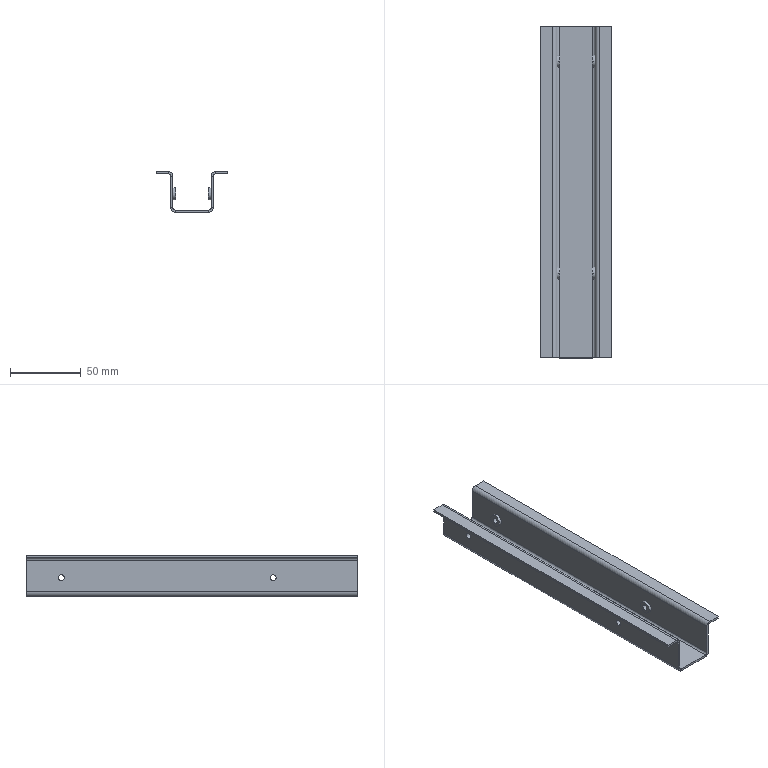Part | SolidWorks | features ICE 2, 3DProfileFeature 1, FlatPattern 1, HoleWzd 1, MirrorPattern 1, SMBaseFlange 1, SheetMetal 1 | 1 solid | 58 faces | box 50 x 235 x 28.5 mm | volume 35580 mm3 | plane 34 | cylinder 24 | commonest cylinder face diameters 4.2 x8 8.7 x8 3 x4 6 x4
STEP:
#1=CARTESIAN_POINT('',(15.,225.,-11.9));
#2=VERTEX_POINT('',#1);
#3=CARTESIAN_POINT('',(15.,225.,-16.1));
#4=VERTEX_POINT('',#3);
#5=CARTESIAN_POINT('',(15.,225.,-14.));
#6=DIRECTION('',(1.,0.,0.));
#7=DIRECTION('',(0.,0.,-1.));
#8=AXIS2_PLACEMENT_3D('',#5,#6,#7);
#9=CIRCLE('',#8,2.1);
#10=EDGE_CURVE('',#2,#4,#9,.T.);
#11=ORIENTED_EDGE('',*,*,#10,.T.);
#12=CARTESIAN_POINT('',(11.5,225.,-16.1));
#13=VERTEX_POINT('',#12);
#14=CARTESIAN_POINT('',(-15.,225.,-16.1));
#15=DIRECTION('',(-1.,0.,0.));
#16=VECTOR('',#15,1000.);
#17=LINE('',#14,#16);
#18=EDGE_CURVE('',#4,#13,#17,.T.);
#19=ORIENTED_EDGE('',*,*,#18,.T.);
#20=CARTESIAN_POINT('',(11.5,225.,-11.9));
#21=VERTEX_POINT('',#20);
#22=CARTESIAN_POINT('',(11.5,225.,-14.));
#23=DIRECTION('',(-1.,0.,0.));
#24=DIRECTION('',(0.,0.,1.));
#25=AXIS2_PLACEMENT_3D('',#22,#23,#24);
#26=CIRCLE('',#25,2.1);
#27=EDGE_CURVE('',#13,#21,#26,.T.);
#28=ORIENTED_EDGE('',*,*,#27,.T.);
#29=CARTESIAN_POINT('',(-15.,225.,-11.9));
#30=DIRECTION('',(-1.,0.,0.));
#31=VECTOR('',#30,1000.);
#32=LINE('',#29,#31);
#33=EDGE_CURVE('',#2,#21,#32,.T.);
#34=ORIENTED_EDGE('',*,*,#33,.F.);
#35=EDGE_LOOP('',(#11,#19,#28,#34));
#36=FACE_OUTER_BOUND('',#35,.T.);
#37=CARTESIAN_POINT('',(-15.,225.,-14.));
#38=DIRECTION('',(-1.,0.,0.));
#39=DIRECTION('',(0.,0.,1.));
#40=AXIS2_PLACEMENT_3D('',#37,#38,#39);
#41=CYLINDRICAL_SURFACE('',#40,2.1);
#42=ADVANCED_FACE('',(#36),#41,.F.);
#43=CARTESIAN_POINT('',(-11.5,225.,-11.9));
#44=VERTEX_POINT('',#43);
#45=CARTESIAN_POINT('',(-11.5,225.,-16.1));
#46=VERTEX_POINT('',#45);
#47=CARTESIAN_POINT('',(-11.5,225.,-14.));
#48=DIRECTION('',(1.,0.,0.));
#49=DIRECTION('',(0.,0.,-1.));
#50=AXIS2_PLACEMENT_3D('',#47,#48,#49);
#51=CIRCLE('',#50,2.1);
#52=EDGE_CURVE('',#44,#46,#51,.T.);
#53=ORIENTED_EDGE('',*,*,#52,.T.);
#54=CARTESIAN_POINT('',(-15.,225.,-16.1));
#55=VERTEX_POINT('',#54);
#56=CARTESIAN_POINT('',(-15.,225.,-16.1));
#57=DIRECTION('',(-1.,0.,0.));
#58=VECTOR('',#57,1000.);
#59=LINE('',#56,#58);
#60=EDGE_CURVE('',#46,#55,#59,.T.);
#61=ORIENTED_EDGE('',*,*,#60,.T.);
#62=CARTESIAN_POINT('',(-15.,225.,-11.9));
#63=VERTEX_POINT('',#62);
#64=CARTESIAN_POINT('',(-15.,225.,-14.));
#65=DIRECTION('',(-1.,0.,0.));
#66=DIRECTION('',(0.,0.,1.));
#67=AXIS2_PLACEMENT_3D('',#64,#65,#66);
#68=CIRCLE('',#67,2.1);
#69=EDGE_CURVE('',#55,#63,#68,.T.);
#70=ORIENTED_EDGE('',*,*,#69,.T.);
#71=CARTESIAN_POINT('',(-15.,225.,-11.9));
#72=DIRECTION('',(-1.,0.,0.));
#73=VECTOR('',#72,1000.);
#74=LINE('',#71,#73);
#75=EDGE_CURVE('',#44,#63,#74,.T.);
#76=ORIENTED_EDGE('',*,*,#75,.F.);
#77=EDGE_LOOP('',(#53,#61,#70,#76));
#78=FACE_OUTER_BOUND('',#77,.T.);
#79=CARTESIAN_POINT('',(-15.,225.,-14.));
#80=DIRECTION('',(-1.,0.,0.));
#81=DIRECTION('',(0.,0.,1.));
#82=AXIS2_PLACEMENT_3D('',#79,#80,#81);
#83=CYLINDRICAL_SURFACE('',#82,2.1);
#84=ADVANCED_FACE('',(#78),#83,.F.);
#85=CARTESIAN_POINT('',(-11.5,75.,-11.9));
#86=VERTEX_POINT('',#85);
#87=CARTESIAN_POINT('',(-11.5,75.,-16.1));
#88=VERTEX_POINT('',#87);
#89=CARTESIAN_POINT('',(-11.5,75.,-14.));
#90=DIRECTION('',(1.,0.,0.));
#91=DIRECTION('',(0.,0.,-1.));
#92=AXIS2_PLACEMENT_3D('',#89,#90,#91);
#93=CIRCLE('',#92,2.1);
#94=EDGE_CURVE('',#86,#88,#93,.T.);
#95=ORIENTED_EDGE('',*,*,#94,.T.);
#96=CARTESIAN_POINT('',(-15.,75.,-16.1));
#97=VERTEX_POINT('',#96);
#98=CARTESIAN_POINT('',(-15.,75.,-16.1));
#99=DIRECTION('',(-1.,0.,0.));
#100=VECTOR('',#99,1000.);
#101=LINE('',#98,#100);
#102=EDGE_CURVE('',#88,#97,#101,.T.);
#103=ORIENTED_EDGE('',*,*,#102,.T.);
#104=CARTESIAN_POINT('',(-15.,75.,-11.9));
#105=VERTEX_POINT('',#104);
#106=CARTESIAN_POINT('',(-15.,75.,-14.));
#107=DIRECTION('',(-1.,0.,0.));
#108=DIRECTION('',(0.,0.,1.));
#109=AXIS2_PLACEMENT_3D('',#106,#107,#108);
#110=CIRCLE('',#109,2.1);
#111=EDGE_CURVE('',#97,#105,#110,.T.);
#112=ORIENTED_EDGE('',*,*,#111,.T.);
#113=CARTESIAN_POINT('',(-15.,75.,-11.9));
#114=DIRECTION('',(-1.,0.,0.));
#115=VECTOR('',#114,1000.);
#116=LINE('',#113,#115);
#117=EDGE_CURVE('',#86,#105,#116,.T.);
#118=ORIENTED_EDGE('',*,*,#117,.F.);
#119=EDGE_LOOP('',(#95,#103,#112,#118));
#120=FACE_OUTER_BOUND('',#119,.T.);
#121=CARTESIAN_POINT('',(-15.,75.,-14.));
#122=DIRECTION('',(-1.,0.,0.));
#123=DIRECTION('',(0.,0.,1.));
#124=AXIS2_PLACEMENT_3D('',#121,#122,#123);
#125=CYLINDRICAL_SURFACE('',#124,2.1);
#126=ADVANCED_FACE('',(#120),#125,.F.);
#127=CARTESIAN_POINT('',(15.,75.,-11.9));
#128=VERTEX_POINT('',#127);
#129=CARTESIAN_POINT('',(15.,75.,-16.1));
#130=VERTEX_POINT('',#129);
#131=CARTESIAN_POINT('',(15.,75.,-14.));
#132=DIRECTION('',(1.,0.,0.));
#133=DIRECTION('',(0.,0.,-1.));
#134=AXIS2_PLACEMENT_3D('',#131,#132,#133);
#135=CIRCLE('',#134,2.1);
#136=EDGE_CURVE('',#128,#130,#135,.T.);
#137=ORIENTED_EDGE('',*,*,#136,.T.);
#138=CARTESIAN_POINT('',(11.5,75.,-16.1));
#139=VERTEX_POINT('',#138);
#140=CARTESIAN_POINT('',(-15.,75.,-16.1));
#141=DIRECTION('',(-1.,0.,0.));
#142=VECTOR('',#141,1000.);
#143=LINE('',#140,#142);
#144=EDGE_CURVE('',#130,#139,#143,.T.);
#145=ORIENTED_EDGE('',*,*,#144,.T.);
#146=CARTESIAN_POINT('',(11.5,75.,-11.9));
#147=VERTEX_POINT('',#146);
#148=CARTESIAN_POINT('',(11.5,75.,-14.));
#149=DIRECTION('',(-1.,0.,0.));
#150=DIRECTION('',(0.,0.,1.));
#151=AXIS2_PLACEMENT_3D('',#148,#149,#150);
#152=CIRCLE('',#151,2.1);
#153=EDGE_CURVE('',#139,#147,#152,.T.);
#154=ORIENTED_EDGE('',*,*,#153,.T.);
#155=CARTESIAN_POINT('',(-15.,75.,-11.9));
#156=DIRECTION('',(-1.,0.,0.));
#157=VECTOR('',#156,1000.);
#158=LINE('',#155,#157);
#159=EDGE_CURVE('',#128,#147,#158,.T.);
#160=ORIENTED_EDGE('',*,*,#159,.F.);
#161=EDGE_LOOP('',(#137,#145,#154,#160));
#162=FACE_OUTER_BOUND('',#161,.T.);
#163=CARTESIAN_POINT('',(-15.,75.,-14.));
#164=DIRECTION('',(-1.,0.,0.));
#165=DIRECTION('',(0.,0.,1.));
#166=AXIS2_PLACEMENT_3D('',#163,#164,#165);
#167=CYLINDRICAL_SURFACE('',#166,2.1);
#168=ADVANCED_FACE('',(#162),#167,.F.);
#169=CARTESIAN_POINT('',(11.5,75.,-18.35));
#170=VERTEX_POINT('',#169);
#171=CARTESIAN_POINT('',(11.5,75.,-9.65));
#172=VERTEX_POINT('',#171);
#173=CARTESIAN_POINT('',(11.5,75.,-14.));
#174=DIRECTION('',(1.,0.,0.));
#175=DIRECTION('',(0.,0.,-1.));
#176=AXIS2_PLACEMENT_3D('',#173,#174,#175);
#177=CIRCLE('',#176,4.35);
#178=EDGE_CURVE('',#170,#172,#177,.T.);
#179=ORIENTED_EDGE('',*,*,#178,.T.);
#180=CARTESIAN_POINT('',(13.5,75.,-9.65));
#181=VERTEX_POINT('',#180);
#182=CARTESIAN_POINT('',(11.5,75.,-9.65));
#183=DIRECTION('',(1.,0.,0.));
#184=VECTOR('',#183,1000.);
#185=LINE('',#182,#184);
#186=EDGE_CURVE('',#172,#181,#185,.T.);
#187=ORIENTED_EDGE('',*,*,#186,.T.);
#188=CARTESIAN_POINT('',(13.5,75.,-18.35));
#189=VERTEX_POINT('',#188);
#190=CARTESIAN_POINT('',(13.5,75.,-14.));
#191=DIRECTION('',(1.,0.,0.));
#192=DIRECTION('',(0.,0.,-1.));
#193=AXIS2_PLACEMENT_3D('',#190,#191,#192);
#194=CIRCLE('',#193,4.35);
#195=EDGE_CURVE('',#189,#181,#194,.T.);
#196=ORIENTED_EDGE('',*,*,#195,.F.);
#197=CARTESIAN_POINT('',(11.5,75.,-18.35));
#198=DIRECTION('',(1.,0.,0.));
#199=VECTOR('',#198,1000.);
#200=LINE('',#197,#199);
#201=EDGE_CURVE('',#170,#189,#200,.T.);
#202=ORIENTED_EDGE('',*,*,#201,.F.);
#203=EDGE_LOOP('',(#179,#187,#196,#202));
#204=FACE_OUTER_BOUND('',#203,.T.);
#205=CARTESIAN_POINT('',(11.5,75.,-14.));
#206=DIRECTION('',(1.,0.,0.));
#207=DIRECTION('',(0.,0.,-1.));
#208=AXIS2_PLACEMENT_3D('',#205,#206,#207);
#209=CYLINDRICAL_SURFACE('',#208,4.35);
#210=ADVANCED_FACE('',(#204),#209,.T.);
#211=CARTESIAN_POINT('',(11.5,225.,-18.35));
#212=VERTEX_POINT('',#211);
#213=CARTESIAN_POINT('',(11.5,225.,-9.65));
#214=VERTEX_POINT('',#213);
#215=CARTESIAN_POINT('',(11.5,225.,-14.));
#216=DIRECTION('',(1.,0.,0.));
#217=DIRECTION('',(0.,0.,-1.));
#218=AXIS2_PLACEMENT_3D('',#215,#216,#217);
#219=CIRCLE('',#218,4.35);
#220=EDGE_CURVE('',#212,#214,#219,.T.);
#221=ORIENTED_EDGE('',*,*,#220,.T.);
#222=CARTESIAN_POINT('',(13.5,225.,-9.65));
#223=VERTEX_POINT('',#222);
#224=CARTESIAN_POINT('',(11.5,225.,-9.65));
#225=DIRECTION('',(1.,0.,0.));
#226=VECTOR('',#225,1000.);
#227=LINE('',#224,#226);
#228=EDGE_CURVE('',#214,#223,#227,.T.);
#229=ORIENTED_EDGE('',*,*,#228,.T.);
#230=CARTESIAN_POINT('',(13.5,225.,-18.35));
#231=VERTEX_POINT('',#230);
#232=CARTESIAN_POINT('',(13.5,225.,-14.));
#233=DIRECTION('',(1.,0.,0.));
#234=DIRECTION('',(0.,0.,-1.));
#235=AXIS2_PLACEMENT_3D('',#232,#233,#234);
#236=CIRCLE('',#235,4.35);
#237=EDGE_CURVE('',#231,#223,#236,.T.);
#238=ORIENTED_EDGE('',*,*,#237,.F.);
#239=CARTESIAN_POINT('',(11.5,225.,-18.35));
#240=DIRECTION('',(1.,0.,0.));
#241=VECTOR('',#240,1000.);
#242=LINE('',#239,#241);
#243=EDGE_CURVE('',#212,#231,#242,.T.);
#244=ORIENTED_EDGE('',*,*,#243,.F.);
#245=EDGE_LOOP('',(#221,#229,#238,#244));
#246=FACE_OUTER_BOUND('',#245,.T.);
#247=CARTESIAN_POINT('',(11.5,225.,-14.));
#248=DIRECTION('',(1.,0.,0.));
#249=DIRECTION('',(0.,0.,-1.));
#250=AXIS2_PLACEMENT_3D('',#247,#248,#249);
#251=CYLINDRICAL_SURFACE('',#250,4.35);
#252=ADVANCED_FACE('',(#246),#251,.T.);
#253=CARTESIAN_POINT('',(-11.5,75.,-18.35));
#254=VERTEX_POINT('',#253);
#255=CARTESIAN_POINT('',(-11.5,75.,-9.65));
#256=VERTEX_POINT('',#255);
#257=CARTESIAN_POINT('',(-11.5,75.,-14.));
#258=DIRECTION('',(1.,0.,0.));
#259=DIRECTION('',(0.,0.,-1.));
#260=AXIS2_PLACEMENT_3D('',#257,#258,#259);
#261=CIRCLE('',#260,4.35);
#262=EDGE_CURVE('',#254,#256,#261,.T.);
#263=ORIENTED_EDGE('',*,*,#262,.F.);
#264=CARTESIAN_POINT('',(-13.5,75.,-18.35));
#265=VERTEX_POINT('',#264);
#266=CARTESIAN_POINT('',(-11.5,75.,-18.35));
#267=DIRECTION('',(-1.,0.,0.));
#268=VECTOR('',#267,1000.);
#269=LINE('',#266,#268);
#270=EDGE_CURVE('',#254,#265,#269,.T.);
#271=ORIENTED_EDGE('',*,*,#270,.T.);
#272=CARTESIAN_POINT('',(-13.5,75.,-9.65));
#273=VERTEX_POINT('',#272);
#274=CARTESIAN_POINT('',(-13.5,75.,-14.));
#275=DIRECTION('',(1.,0.,0.));
#276=DIRECTION('',(0.,0.,1.));
#277=AXIS2_PLACEMENT_3D('',#274,#275,#276);
#278=CIRCLE('',#277,4.35);
#279=EDGE_CURVE('',#265,#273,#278,.T.);
#280=ORIENTED_EDGE('',*,*,#279,.T.);
#281=CARTESIAN_POINT('',(-11.5,75.,-9.65));
#282=DIRECTION('',(-1.,0.,0.));
#283=VECTOR('',#282,1000.);
#284=LINE('',#281,#283);
#285=EDGE_CURVE('',#256,#273,#284,.T.);
#286=ORIENTED_EDGE('',*,*,#285,.F.);
#287=EDGE_LOOP('',(#263,#271,#280,#286));
#288=FACE_OUTER_BOUND('',#287,.T.);
#289=CARTESIAN_POINT('',(-11.5,75.,-14.));
#290=DIRECTION('',(-1.,0.,0.));
#291=DIRECTION('',(0.,0.,1.));
#292=AXIS2_PLACEMENT_3D('',#289,#290,#291);
#293=CYLINDRICAL_SURFACE('',#292,4.35);
#294=ADVANCED_FACE('',(#288),#293,.T.);
#295=CARTESIAN_POINT('',(-11.5,225.,-18.35));
#296=VERTEX_POINT('',#295);
#297=CARTESIAN_POINT('',(-11.5,225.,-9.65));
#298=VERTEX_POINT('',#297);
#299=CARTESIAN_POINT('',(-11.5,225.,-14.));
#300=DIRECTION('',(1.,0.,0.));
#301=DIRECTION('',(0.,0.,-1.));
#302=AXIS2_PLACEMENT_3D('',#299,#300,#301);
#303=CIRCLE('',#302,4.35);
#304=EDGE_CURVE('',#296,#298,#303,.T.);
#305=ORIENTED_EDGE('',*,*,#304,.F.);
#306=CARTESIAN_POINT('',(-13.5,225.,-18.35));
#307=VERTEX_POINT('',#306);
#308=CARTESIAN_POINT('',(-11.5,225.,-18.35));
#309=DIRECTION('',(-1.,0.,0.));
#310=VECTOR('',#309,1000.);
#311=LINE('',#308,#310);
#312=EDGE_CURVE('',#296,#307,#311,.T.);
#313=ORIENTED_EDGE('',*,*,#312,.T.);
#314=CARTESIAN_POINT('',(-13.5,225.,-9.65));
#315=VERTEX_POINT('',#314);
#316=CARTESIAN_POINT('',(-13.5,225.,-14.));
#317=DIRECTION('',(1.,0.,0.));
#318=DIRECTION('',(0.,0.,1.));
#319=AXIS2_PLACEMENT_3D('',#316,#317,#318);
#320=CIRCLE('',#319,4.35);
#321=EDGE_CURVE('',#307,#315,#320,.T.);
#322=ORIENTED_EDGE('',*,*,#321,.T.);
#323=CARTESIAN_POINT('',(-11.5,225.,-9.65));
#324=DIRECTION('',(-1.,0.,0.));
#325=VECTOR('',#324,1000.);
#326=LINE('',#323,#325);
#327=EDGE_CURVE('',#298,#315,#326,.T.);
#328=ORIENTED_EDGE('',*,*,#327,.F.);
#329=EDGE_LOOP('',(#305,#313,#322,#328));
#330=FACE_OUTER_BOUND('',#329,.T.);
#331=CARTESIAN_POINT('',(-11.5,225.,-14.));
#332=DIRECTION('',(-1.,0.,0.));
#333=DIRECTION('',(0.,0.,1.));
#334=AXIS2_PLACEMENT_3D('',#331,#332,#333);
#335=CYLINDRICAL_SURFACE('',#334,4.35);
#336=ADVANCED_FACE('',(#330),#335,.T.);
#337=CARTESIAN_POINT('',(-25.,15.,0.));
#338=VERTEX_POINT('',#337);
#339=CARTESIAN_POINT('',(-16.5,15.,0.));
#340=VERTEX_POINT('',#339);
#341=CARTESIAN_POINT('',(-25.,15.,0.));
#342=DIRECTION('',(1.,0.,0.));
#343=VECTOR('',#342,1000.);
#344=LINE('',#341,#343);
#345=EDGE_CURVE('',#338,#340,#344,.T.);
#346=ORIENTED_EDGE('',*,*,#345,.T.);
#347=CARTESIAN_POINT('',(-16.5,15.,1.5));
#348=VERTEX_POINT('',#347);
#349=CARTESIAN_POINT('',(-16.5,15.,0.));
#350=DIRECTION('',(0.,0.,1.));
#351=VECTOR('',#350,1000.);
#352=LINE('',#349,#351);
#353=EDGE_CURVE('',#340,#348,#352,.T.);
#354=ORIENTED_EDGE('',*,*,#353,.T.);
#355=CARTESIAN_POINT('',(-25.,15.,1.5));
#356=VERTEX_POINT('',#355);
#357=CARTESIAN_POINT('',(-25.,15.,1.5));
#358=DIRECTION('',(1.,0.,0.));
#359=VECTOR('',#358,1000.);
#360=LINE('',#357,#359);
#361=EDGE_CURVE('',#356,#348,#360,.T.);
#362=ORIENTED_EDGE('',*,*,#361,.F.);
#363=CARTESIAN_POINT('',(-25.,15.,-43.176));
#364=DIRECTION('',(0.,0.,-1.));
#365=VECTOR('',#364,1000.);
#366=LINE('',#363,#365);
#367=EDGE_CURVE('',#356,#338,#366,.T.);
#368=ORIENTED_EDGE('',*,*,#367,.T.);
#369=EDGE_LOOP('',(#346,#354,#362,#368));
#370=FACE_OUTER_BOUND('',#369,.T.);
#371=CARTESIAN_POINT('',(25.,15.,-43.176));
#372=DIRECTION('',(0.,1.,0.));
#373=DIRECTION('',(0.,0.,1.));
#374=AXIS2_PLACEMENT_3D('',#371,#372,#373);
#375=PLANE('',#374);
#376=ADVANCED_FACE('',(#370),#375,.F.);
#377=CARTESIAN_POINT('',(-13.5,15.,-1.5));
#378=VERTEX_POINT('',#377);
#379=CARTESIAN_POINT('',(-13.5,15.,-24.));
#380=VERTEX_POINT('',#379);
#381=CARTESIAN_POINT('',(-13.5,15.,0.));
#382=DIRECTION('',(0.,0.,-1.));
#383=VECTOR('',#382,1000.);
#384=LINE('',#381,#383);
#385=EDGE_CURVE('',#378,#380,#384,.T.);
#386=ORIENTED_EDGE('',*,*,#385,.F.);
#387=CARTESIAN_POINT('',(-15.,15.,-1.5));
#388=VERTEX_POINT('',#387);
#389=CARTESIAN_POINT('',(-13.5,15.,-1.5));
#390=DIRECTION('',(-1.,0.,0.));
#391=VECTOR('',#390,1000.);
#392=LINE('',#389,#391);
#393=EDGE_CURVE('',#378,#388,#392,.T.);
#394=ORIENTED_EDGE('',*,*,#393,.T.);
#395=CARTESIAN_POINT('',(-15.,15.,-24.));
#396=VERTEX_POINT('',#395);
#397=CARTESIAN_POINT('',(-15.,15.,0.));
#398=DIRECTION('',(0.,0.,-1.));
#399=VECTOR('',#398,1000.);
#400=LINE('',#397,#399);
#401=EDGE_CURVE('',#388,#396,#400,.T.);
#402=ORIENTED_EDGE('',*,*,#401,.T.);
#403=CARTESIAN_POINT('',(-15.,15.,-24.));
#404=DIRECTION('',(1.,0.,0.));
#405=VECTOR('',#404,1000.);
#406=LINE('',#403,#405);
#407=EDGE_CURVE('',#396,#380,#406,.T.);
#408=ORIENTED_EDGE('',*,*,#407,.T.);
#409=EDGE_LOOP('',(#386,#394,#402,#408));
#410=FACE_OUTER_BOUND('',#409,.T.);
#411=CARTESIAN_POINT('',(25.,15.,-43.176));
#412=DIRECTION('',(0.,1.,0.));
#413=DIRECTION('',(0.,0.,1.));
#414=AXIS2_PLACEMENT_3D('',#411,#412,#413);
#415=PLANE('',#414);
#416=ADVANCED_FACE('',(#410),#415,.F.);
#417=ORIENTED_EDGE('',*,*,#353,.F.);
#418=CARTESIAN_POINT('',(-16.5,15.,-1.5));
#419=DIRECTION('',(0.,1.,0.));
#420=DIRECTION('',(0.,0.,1.));
#421=AXIS2_PLACEMENT_3D('',#418,#419,#420);
#422=CIRCLE('',#421,1.5);
#423=EDGE_CURVE('',#340,#388,#422,.T.);
#424=ORIENTED_EDGE('',*,*,#423,.T.);
#425=ORIENTED_EDGE('',*,*,#393,.F.);
#426=CARTESIAN_POINT('',(-16.5,15.,-1.5));
#427=DIRECTION('',(0.,1.,0.));
#428=DIRECTION('',(0.,0.,1.));
#429=AXIS2_PLACEMENT_3D('',#426,#427,#428);
#430=CIRCLE('',#429,3.);
#431=EDGE_CURVE('',#348,#378,#430,.T.);
#432=ORIENTED_EDGE('',*,*,#431,.F.);
#433=EDGE_LOOP('',(#417,#424,#425,#432));
#434=FACE_OUTER_BOUND('',#433,.T.);
#435=CARTESIAN_POINT('',(25.,15.,-43.176));
#436=DIRECTION('',(0.,1.,0.));
#437=DIRECTION('',(0.,0.,1.));
#438=AXIS2_PLACEMENT_3D('',#435,#436,#437);
#439=PLANE('',#438);
#440=ADVANCED_FACE('',(#434),#439,.F.);
#441=CARTESIAN_POINT('',(-12.,15.,-25.5));
#442=VERTEX_POINT('',#441);
#443=CARTESIAN_POINT('',(12.,15.,-25.5));
#444=VERTEX_POINT('',#443);
#445=CARTESIAN_POINT('',(-15.,15.,-25.5));
#446=DIRECTION('',(1.,0.,0.));
#447=VECTOR('',#446,1000.);
#448=LINE('',#445,#447);
#449=EDGE_CURVE('',#442,#444,#448,.T.);
#450=ORIENTED_EDGE('',*,*,#449,.F.);
#451=CARTESIAN_POINT('',(-12.,15.,-27.));
#452=VERTEX_POINT('',#451);
#453=CARTESIAN_POINT('',(-12.,15.,-25.5));
#454=DIRECTION('',(0.,0.,-1.));
#455=VECTOR('',#454,1000.);
#456=LINE('',#453,#455);
#457=EDGE_CURVE('',#442,#452,#456,.T.);
#458=ORIENTED_EDGE('',*,*,#457,.T.);
#459=CARTESIAN_POINT('',(12.,15.,-27.));
#460=VERTEX_POINT('',#459);
#461=CARTESIAN_POINT('',(-15.,15.,-27.));
#462=DIRECTION('',(1.,0.,0.));
#463=VECTOR('',#462,1000.);
#464=LINE('',#461,#463);
#465=EDGE_CURVE('',#452,#460,#464,.T.);
#466=ORIENTED_EDGE('',*,*,#465,.T.);
#467=CARTESIAN_POINT('',(12.,15.,-27.));
#468=DIRECTION('',(0.,0.,1.));
#469=VECTOR('',#468,1000.);
#470=LINE('',#467,#469);
#471=EDGE_CURVE('',#460,#444,#470,.T.);
#472=ORIENTED_EDGE('',*,*,#471,.T.);
#473=EDGE_LOOP('',(#450,#458,#466,#472));
#474=FACE_OUTER_BOUND('',#473,.T.);
#475=CARTESIAN_POINT('',(25.,15.,-43.176));
#476=DIRECTION('',(0.,1.,0.));
#477=DIRECTION('',(0.,0.,1.));
#478=AXIS2_PLACEMENT_3D('',#475,#476,#477);
#479=PLANE('',#478);
#480=ADVANCED_FACE('',(#474),#479,.F.);
#481=ORIENTED_EDGE('',*,*,#407,.F.);
#482=CARTESIAN_POINT('',(-12.,15.,-24.));
#483=DIRECTION('',(0.,-1.,0.));
#484=DIRECTION('',(0.,0.,1.));
#485=AXIS2_PLACEMENT_3D('',#482,#483,#484);
#486=CIRCLE('',#485,3.);
#487=EDGE_CURVE('',#396,#452,#486,.T.);
#488=ORIENTED_EDGE('',*,*,#487,.T.);
#489=ORIENTED_EDGE('',*,*,#457,.F.);
#490=CARTESIAN_POINT('',(-12.,15.,-24.));
#491=DIRECTION('',(0.,-1.,0.));
#492=DIRECTION('',(0.,0.,1.));
#493=AXIS2_PLACEMENT_3D('',#490,#491,#492);
#494=CIRCLE('',#493,1.5);
#495=EDGE_CURVE('',#380,#442,#494,.T.);
#496=ORIENTED_EDGE('',*,*,#495,.F.);
#497=EDGE_LOOP('',(#481,#488,#489,#496));
#498=FACE_OUTER_BOUND('',#497,.T.);
#499=CARTESIAN_POINT('',(25.,15.,-43.176));
#500=DIRECTION('',(0.,1.,0.));
#501=DIRECTION('',(0.,0.,1.));
#502=AXIS2_PLACEMENT_3D('',#499,#500,#501);
#503=PLANE('',#502);
#504=ADVANCED_FACE('',(#498),#503,.F.);
#505=CARTESIAN_POINT('',(13.5,15.,-24.));
#506=VERTEX_POINT('',#505);
#507=CARTESIAN_POINT('',(13.5,15.,-1.5));
#508=VERTEX_POINT('',#507);
#509=CARTESIAN_POINT('',(13.5,15.,-27.));
#510=DIRECTION('',(0.,0.,1.));
#511=VECTOR('',#510,1000.);
#512=LINE('',#509,#511);
#513=EDGE_CURVE('',#506,#508,#512,.T.);
#514=ORIENTED_EDGE('',*,*,#513,.F.);
#515=CARTESIAN_POINT('',(15.,15.,-24.));
#516=VERTEX_POINT('',#515);
#517=CARTESIAN_POINT('',(13.5,15.,-24.));
#518=DIRECTION('',(1.,0.,0.));
#519=VECTOR('',#518,1000.);
#520=LINE('',#517,#519);
#521=EDGE_CURVE('',#506,#516,#520,.T.);
#522=ORIENTED_EDGE('',*,*,#521,.T.);
#523=CARTESIAN_POINT('',(15.,15.,-1.5));
#524=VERTEX_POINT('',#523);
#525=CARTESIAN_POINT('',(15.,15.,-27.));
#526=DIRECTION('',(0.,0.,1.));
#527=VECTOR('',#526,1000.);
#528=LINE('',#525,#527);
#529=EDGE_CURVE('',#516,#524,#528,.T.);
#530=ORIENTED_EDGE('',*,*,#529,.T.);
#531=CARTESIAN_POINT('',(15.,15.,-1.5));
#532=DIRECTION('',(-1.,0.,0.));
#533=VECTOR('',#532,1000.);
#534=LINE('',#531,#533);
#535=EDGE_CURVE('',#524,#508,#534,.T.);
#536=ORIENTED_EDGE('',*,*,#535,.T.);
#537=EDGE_LOOP('',(#514,#522,#530,#536));
#538=FACE_OUTER_BOUND('',#537,.T.);
#539=CARTESIAN_POINT('',(25.,15.,-43.176));
#540=DIRECTION('',(0.,1.,0.));
#541=DIRECTION('',(0.,0.,1.));
#542=AXIS2_PLACEMENT_3D('',#539,#540,#541);
#543=PLANE('',#542);
#544=ADVANCED_FACE('',(#538),#543,.F.);
#545=ORIENTED_EDGE('',*,*,#471,.F.);
#546=CARTESIAN_POINT('',(12.,15.,-24.));
#547=DIRECTION('',(0.,-1.,0.));
#548=DIRECTION('',(0.,0.,1.));
#549=AXIS2_PLACEMENT_3D('',#546,#547,#548);
#550=CIRCLE('',#549,3.);
#551=EDGE_CURVE('',#460,#516,#550,.T.);
#552=ORIENTED_EDGE('',*,*,#551,.T.);
#553=ORIENTED_EDGE('',*,*,#521,.F.);
#554=CARTESIAN_POINT('',(12.,15.,-24.));
#555=DIRECTION('',(0.,-1.,0.));
#556=DIRECTION('',(0.,0.,1.));
#557=AXIS2_PLACEMENT_3D('',#554,#555,#556);
#558=CIRCLE('',#557,1.5);
#559=EDGE_CURVE('',#444,#506,#558,.T.);
#560=ORIENTED_EDGE('',*,*,#559,.F.);
#561=EDGE_LOOP('',(#545,#552,#553,#560));
#562=FACE_OUTER_BOUND('',#561,.T.);
#563=CARTESIAN_POINT('',(25.,15.,-43.176));
#564=DIRECTION('',(0.,1.,0.));
#565=DIRECTION('',(0.,0.,1.));
#566=AXIS2_PLACEMENT_3D('',#563,#564,#565);
#567=PLANE('',#566);
#568=ADVANCED_FACE('',(#562),#567,.F.);
#569=CARTESIAN_POINT('',(16.5,15.,1.5));
#570=VERTEX_POINT('',#569);
#571=CARTESIAN_POINT('',(25.,15.,1.5));
#572=VERTEX_POINT('',#571);
#573=CARTESIAN_POINT('',(15.,15.,1.5));
#574=DIRECTION('',(1.,0.,0.));
#575=VECTOR('',#574,1000.);
#576=LINE('',#573,#575);
#577=EDGE_CURVE('',#570,#572,#576,.T.);
#578=ORIENTED_EDGE('',*,*,#577,.F.);
#579=CARTESIAN_POINT('',(16.5,15.,0.));
#580=VERTEX_POINT('',#579);
#581=CARTESIAN_POINT('',(16.5,15.,1.5));
#582=DIRECTION('',(0.,0.,-1.));
#583=VECTOR('',#582,1000.);
#584=LINE('',#581,#583);
#585=EDGE_CURVE('',#570,#580,#584,.T.);
#586=ORIENTED_EDGE('',*,*,#585,.T.);
#587=CARTESIAN_POINT('',(25.,15.,0.));
#588=VERTEX_POINT('',#587);
#589=CARTESIAN_POINT('',(15.,15.,0.));
#590=DIRECTION('',(1.,0.,0.));
#591=VECTOR('',#590,1000.);
#592=LINE('',#589,#591);
#593=EDGE_CURVE('',#580,#588,#592,.T.);
#594=ORIENTED_EDGE('',*,*,#593,.T.);
#595=CARTESIAN_POINT('',(25.,15.,-43.176));
#596=DIRECTION('',(0.,0.,-1.));
#597=VECTOR('',#596,1000.);
#598=LINE('',#595,#597);
#599=EDGE_CURVE('',#572,#588,#598,.T.);
#600=ORIENTED_EDGE('',*,*,#599,.F.);
#601=EDGE_LOOP('',(#578,#586,#594,#600));
#602=FACE_OUTER_BOUND('',#601,.T.);
#603=CARTESIAN_POINT('',(25.,15.,-43.176));
#604=DIRECTION('',(0.,1.,0.));
#605=DIRECTION('',(0.,0.,1.));
#606=AXIS2_PLACEMENT_3D('',#603,#604,#605);
#607=PLANE('',#606);
#608=ADVANCED_FACE('',(#602),#607,.F.);
#609=CARTESIAN_POINT('',(-15.,250.,-1.5));
#610=VERTEX_POINT('',#609);
#611=CARTESIAN_POINT('',(-13.5,250.,-1.5));
#612=VERTEX_POINT('',#611);
#613=CARTESIAN_POINT('',(-15.,250.,-1.5));
#614=DIRECTION('',(1.,0.,0.));
#615=VECTOR('',#614,1000.);
#616=LINE('',#613,#615);
#617=EDGE_CURVE('',#610,#612,#616,.T.);
#618=ORIENTED_EDGE('',*,*,#617,.F.);
#619=CARTESIAN_POINT('',(-16.5,250.,0.));
#620=VERTEX_POINT('',#619);
#621=CARTESIAN_POINT('',(-16.5,250.,-1.5));
#622=DIRECTION('',(0.,1.,0.));
#623=DIRECTION('',(0.,0.,-1.));
#624=AXIS2_PLACEMENT_3D('',#621,#622,#623);
#625=CIRCLE('',#624,1.5);
#626=EDGE_CURVE('',#620,#610,#625,.T.);
#627=ORIENTED_EDGE('',*,*,#626,.F.);
#628=CARTESIAN_POINT('',(-16.5,250.,1.5));
#629=VERTEX_POINT('',#628);
#630=CARTESIAN_POINT('',(-16.5,250.,1.5));
#631=DIRECTION('',(0.,0.,-1.));
#632=VECTOR('',#631,1000.);
#633=LINE('',#630,#632);
#634=EDGE_CURVE('',#629,#620,#633,.T.);
#635=ORIENTED_EDGE('',*,*,#634,.F.);
#636=CARTESIAN_POINT('',(-16.5,250.,-1.5));
#637=DIRECTION('',(0.,1.,0.));
#638=DIRECTION('',(1.,0.,0.));
#639=AXIS2_PLACEMENT_3D('',#636,#637,#638);
#640=CIRCLE('',#639,3.);
#641=EDGE_CURVE('',#629,#612,#640,.T.);
#642=ORIENTED_EDGE('',*,*,#641,.T.);
#643=EDGE_LOOP('',(#618,#627,#635,#642));
#644=FACE_OUTER_BOUND('',#643,.T.);
#645=CARTESIAN_POINT('',(-15.,250.,-1.5));
#646=DIRECTION('',(0.,1.,0.));
#647=DIRECTION('',(0.,0.,1.));
#648=AXIS2_PLACEMENT_3D('',#645,#646,#647);
#649=PLANE('',#648);
#650=ADVANCED_FACE('',(#644),#649,.T.);
#651=CARTESIAN_POINT('',(-15.,250.,-24.));
#652=VERTEX_POINT('',#651);
#653=CARTESIAN_POINT('',(-15.,250.,0.));
#654=DIRECTION('',(0.,0.,-1.));
#655=VECTOR('',#654,1000.);
#656=LINE('',#653,#655);
#657=EDGE_CURVE('',#610,#652,#656,.T.);
#658=ORIENTED_EDGE('',*,*,#657,.F.);
#659=ORIENTED_EDGE('',*,*,#617,.T.);
#660=CARTESIAN_POINT('',(-13.5,250.,-24.));
#661=VERTEX_POINT('',#660);
#662=CARTESIAN_POINT('',(-13.5,250.,0.));
#663=DIRECTION('',(0.,0.,-1.));
#664=VECTOR('',#663,1000.);
#665=LINE('',#662,#664);
#666=EDGE_CURVE('',#612,#661,#665,.T.);
#667=ORIENTED_EDGE('',*,*,#666,.T.);
#668=CARTESIAN_POINT('',(-13.5,250.,-24.));
#669=DIRECTION('',(-1.,0.,0.));
#670=VECTOR('',#669,1000.);
#671=LINE('',#668,#670);
#672=EDGE_CURVE('',#661,#652,#671,.T.);
#673=ORIENTED_EDGE('',*,*,#672,.T.);
#674=EDGE_LOOP('',(#658,#659,#667,#673));
#675=FACE_OUTER_BOUND('',#674,.T.);
#676=CARTESIAN_POINT('',(-16.5,250.,1.5));
#677=DIRECTION('',(0.,1.,0.));
#678=DIRECTION('',(0.,0.,1.));
#679=AXIS2_PLACEMENT_3D('',#676,#677,#678);
#680=PLANE('',#679);
#681=ADVANCED_FACE('',(#675),#680,.T.);
#682=CARTESIAN_POINT('',(-12.,250.,-27.));
#683=VERTEX_POINT('',#682);
#684=CARTESIAN_POINT('',(-12.,250.,-25.5));
#685=VERTEX_POINT('',#684);
#686=CARTESIAN_POINT('',(-12.,250.,-27.));
#687=DIRECTION('',(0.,0.,1.));
#688=VECTOR('',#687,1000.);
#689=LINE('',#686,#688);
#690=EDGE_CURVE('',#683,#685,#689,.T.);
#691=ORIENTED_EDGE('',*,*,#690,.F.);
#692=CARTESIAN_POINT('',(-12.,250.,-24.));
#693=DIRECTION('',(0.,-1.,0.));
#694=DIRECTION('',(0.,0.,1.));
#695=AXIS2_PLACEMENT_3D('',#692,#693,#694);
#696=CIRCLE('',#695,3.);
#697=EDGE_CURVE('',#652,#683,#696,.T.);
#698=ORIENTED_EDGE('',*,*,#697,.F.);
#699=ORIENTED_EDGE('',*,*,#672,.F.);
#700=CARTESIAN_POINT('',(-12.,250.,-24.));
#701=DIRECTION('',(0.,-1.,0.));
#702=DIRECTION('',(1.,0.,0.));
#703=AXIS2_PLACEMENT_3D('',#700,#701,#702);
#704=CIRCLE('',#703,1.5);
#705=EDGE_CURVE('',#661,#685,#704,.T.);
#706=ORIENTED_EDGE('',*,*,#705,.T.);
#707=EDGE_LOOP('',(#691,#698,#699,#706));
#708=FACE_OUTER_BOUND('',#707,.T.);
#709=CARTESIAN_POINT('',(-12.,250.,-27.));
#710=DIRECTION('',(0.,1.,0.));
#711=DIRECTION('',(0.,0.,1.));
#712=AXIS2_PLACEMENT_3D('',#709,#710,#711);
#713=PLANE('',#712);
#714=ADVANCED_FACE('',(#708),#713,.T.);
#715=CARTESIAN_POINT('',(12.,250.,-27.));
#716=VERTEX_POINT('',#715);
#717=CARTESIAN_POINT('',(-15.,250.,-27.));
#718=DIRECTION('',(1.,0.,0.));
#719=VECTOR('',#718,1000.);
#720=LINE('',#717,#719);
#721=EDGE_CURVE('',#683,#716,#720,.T.);
#722=ORIENTED_EDGE('',*,*,#721,.F.);
#723=ORIENTED_EDGE('',*,*,#690,.T.);
#724=CARTESIAN_POINT('',(12.,250.,-25.5));
#725=VERTEX_POINT('',#724);
#726=CARTESIAN_POINT('',(-15.,250.,-25.5));
#727=DIRECTION('',(1.,0.,0.));
#728=VECTOR('',#727,1000.);
#729=LINE('',#726,#728);
#730=EDGE_CURVE('',#685,#725,#729,.T.);
#731=ORIENTED_EDGE('',*,*,#730,.T.);
#732=CARTESIAN_POINT('',(12.,250.,-25.5));
#733=DIRECTION('',(0.,0.,-1.));
#734=VECTOR('',#733,1000.);
#735=LINE('',#732,#734);
#736=EDGE_CURVE('',#725,#716,#735,.T.);
#737=ORIENTED_EDGE('',*,*,#736,.T.);
#738=EDGE_LOOP('',(#722,#723,#731,#737));
#739=FACE_OUTER_BOUND('',#738,.T.);
#740=CARTESIAN_POINT('',(-13.5,250.,-24.));
#741=DIRECTION('',(0.,1.,0.));
#742=DIRECTION('',(0.,0.,1.));
#743=AXIS2_PLACEMENT_3D('',#740,#741,#742);
#744=PLANE('',#743);
#745=ADVANCED_FACE('',(#739),#744,.T.);
#746=CARTESIAN_POINT('',(15.,250.,-24.));
#747=VERTEX_POINT('',#746);
#748=CARTESIAN_POINT('',(13.5,250.,-24.));
#749=VERTEX_POINT('',#748);
#750=CARTESIAN_POINT('',(15.,250.,-24.));
#751=DIRECTION('',(-1.,0.,0.));
#752=VECTOR('',#751,1000.);
#753=LINE('',#750,#752);
#754=EDGE_CURVE('',#747,#749,#753,.T.);
#755=ORIENTED_EDGE('',*,*,#754,.F.);
#756=CARTESIAN_POINT('',(12.,250.,-24.));
#757=DIRECTION('',(0.,-1.,0.));
#758=DIRECTION('',(0.,0.,1.));
#759=AXIS2_PLACEMENT_3D('',#756,#757,#758);
#760=CIRCLE('',#759,3.);
#761=EDGE_CURVE('',#716,#747,#760,.T.);
#762=ORIENTED_EDGE('',*,*,#761,.F.);
#763=ORIENTED_EDGE('',*,*,#736,.F.);
#764=CARTESIAN_POINT('',(12.,250.,-24.));
#765=DIRECTION('',(0.,-1.,0.));
#766=DIRECTION('',(1.,0.,0.));
#767=AXIS2_PLACEMENT_3D('',#764,#765,#766);
#768=CIRCLE('',#767,1.5);
#769=EDGE_CURVE('',#725,#749,#768,.T.);
#770=ORIENTED_EDGE('',*,*,#769,.T.);
#771=EDGE_LOOP('',(#755,#762,#763,#770));
#772=FACE_OUTER_BOUND('',#771,.T.);
#773=CARTESIAN_POINT('',(15.,250.,-24.));
#774=DIRECTION('',(0.,1.,0.));
#775=DIRECTION('',(0.,0.,1.));
#776=AXIS2_PLACEMENT_3D('',#773,#774,#775);
#777=PLANE('',#776);
#778=ADVANCED_FACE('',(#772),#777,.T.);
#779=CARTESIAN_POINT('',(15.,250.,-1.5));
#780=VERTEX_POINT('',#779);
#781=CARTESIAN_POINT('',(15.,250.,-27.));
#782=DIRECTION('',(0.,0.,1.));
#783=VECTOR('',#782,1000.);
#784=LINE('',#781,#783);
#785=EDGE_CURVE('',#747,#780,#784,.T.);
#786=ORIENTED_EDGE('',*,*,#785,.F.);
#787=ORIENTED_EDGE('',*,*,#754,.T.);
#788=CARTESIAN_POINT('',(13.5,250.,-1.5));
#789=VERTEX_POINT('',#788);
#790=CARTESIAN_POINT('',(13.5,250.,-27.));
#791=DIRECTION('',(0.,0.,1.));
#792=VECTOR('',#791,1000.);
#793=LINE('',#790,#792);
#794=EDGE_CURVE('',#749,#789,#793,.T.);
#795=ORIENTED_EDGE('',*,*,#794,.T.);
#796=CARTESIAN_POINT('',(13.5,250.,-1.5));
#797=DIRECTION('',(1.,0.,0.));
#798=VECTOR('',#797,1000.);
#799=LINE('',#796,#798);
#800=EDGE_CURVE('',#789,#780,#799,.T.);
#801=ORIENTED_EDGE('',*,*,#800,.T.);
#802=EDGE_LOOP('',(#786,#787,#795,#801));
#803=FACE_OUTER_BOUND('',#802,.T.);
#804=CARTESIAN_POINT('',(12.,250.,-25.5));
#805=DIRECTION('',(0.,1.,0.));
#806=DIRECTION('',(0.,0.,1.));
#807=AXIS2_PLACEMENT_3D('',#804,#805,#806);
#808=PLANE('',#807);
#809=ADVANCED_FACE('',(#803),#808,.T.);
#810=CARTESIAN_POINT('',(16.5,250.,0.));
#811=VERTEX_POINT('',#810);
#812=CARTESIAN_POINT('',(16.5,250.,1.5));
#813=VERTEX_POINT('',#812);
#814=CARTESIAN_POINT('',(16.5,250.,0.));
#815=DIRECTION('',(0.,0.,1.));
#816=VECTOR('',#815,1000.);
#817=LINE('',#814,#816);
#818=EDGE_CURVE('',#811,#813,#817,.T.);
#819=ORIENTED_EDGE('',*,*,#818,.F.);
#820=CARTESIAN_POINT('',(16.5,250.,-1.5));
#821=DIRECTION('',(0.,1.,0.));
#822=DIRECTION('',(0.,0.,-1.));
#823=AXIS2_PLACEMENT_3D('',#820,#821,#822);
#824=CIRCLE('',#823,1.5);
#825=EDGE_CURVE('',#780,#811,#824,.T.);
#826=ORIENTED_EDGE('',*,*,#825,.F.);
#827=ORIENTED_EDGE('',*,*,#800,.F.);
#828=CARTESIAN_POINT('',(16.5,250.,-1.5));
#829=DIRECTION('',(0.,1.,0.));
#830=DIRECTION('',(1.,0.,0.));
#831=AXIS2_PLACEMENT_3D('',#828,#829,#830);
#832=CIRCLE('',#831,3.);
#833=EDGE_CURVE('',#789,#813,#832,.T.);
#834=ORIENTED_EDGE('',*,*,#833,.T.);
#835=EDGE_LOOP('',(#819,#826,#827,#834));
#836=FACE_OUTER_BOUND('',#835,.T.);
#837=CARTESIAN_POINT('',(16.5,250.,0.));
#838=DIRECTION('',(0.,1.,0.));
#839=DIRECTION('',(0.,0.,1.));
#840=AXIS2_PLACEMENT_3D('',#837,#838,#839);
#841=PLANE('',#840);
#842=ADVANCED_FACE('',(#836),#841,.T.);
#843=CARTESIAN_POINT('',(25.,250.,0.));
#844=VERTEX_POINT('',#843);
#845=CARTESIAN_POINT('',(15.,250.,0.));
#846=DIRECTION('',(1.,0.,0.));
#847=VECTOR('',#846,1000.);
#848=LINE('',#845,#847);
#849=EDGE_CURVE('',#811,#844,#848,.T.);
#850=ORIENTED_EDGE('',*,*,#849,.F.);
#851=ORIENTED_EDGE('',*,*,#818,.T.);
#852=CARTESIAN_POINT('',(25.,250.,1.5));
#853=VERTEX_POINT('',#852);
#854=CARTESIAN_POINT('',(15.,250.,1.5));
#855=DIRECTION('',(1.,0.,0.));
#856=VECTOR('',#855,1000.);
#857=LINE('',#854,#856);
#858=EDGE_CURVE('',#813,#853,#857,.T.);
#859=ORIENTED_EDGE('',*,*,#858,.T.);
#860=CARTESIAN_POINT('',(25.,250.,0.));
#861=DIRECTION('',(0.,0.,1.));
#862=VECTOR('',#861,1000.);
#863=LINE('',#860,#862);
#864=EDGE_CURVE('',#844,#853,#863,.T.);
#865=ORIENTED_EDGE('',*,*,#864,.F.);
#866=EDGE_LOOP('',(#850,#851,#859,#865));
#867=FACE_OUTER_BOUND('',#866,.T.);
#868=CARTESIAN_POINT('',(13.5,250.,-1.5));
#869=DIRECTION('',(0.,1.,0.));
#870=DIRECTION('',(0.,0.,1.));
#871=AXIS2_PLACEMENT_3D('',#868,#869,#870);
#872=PLANE('',#871);
#873=ADVANCED_FACE('',(#867),#872,.T.);
#874=CARTESIAN_POINT('',(16.5,250.,1.5));
#875=DIRECTION('',(0.,-1.,0.));
#876=VECTOR('',#875,1000.);
#877=LINE('',#874,#876);
#878=EDGE_CURVE('',#813,#570,#877,.T.);
#879=ORIENTED_EDGE('',*,*,#878,.T.);
#880=ORIENTED_EDGE('',*,*,#577,.T.);
#881=CARTESIAN_POINT('',(25.,250.,1.5));
#882=DIRECTION('',(0.,-1.,0.));
#883=VECTOR('',#882,1000.);
#884=LINE('',#881,#883);
#885=EDGE_CURVE('',#853,#572,#884,.T.);
#886=ORIENTED_EDGE('',*,*,#885,.F.);
#887=ORIENTED_EDGE('',*,*,#858,.F.);
#888=EDGE_LOOP('',(#879,#880,#886,#887));
#889=FACE_OUTER_BOUND('',#888,.T.);
#890=CARTESIAN_POINT('',(15.,250.,1.5));
#891=DIRECTION('',(0.,0.,-1.));
#892=DIRECTION('',(-1.,0.,0.));
#893=AXIS2_PLACEMENT_3D('',#890,#891,#892);
#894=PLANE('',#893);
#895=ADVANCED_FACE('',(#889),#894,.F.);
#896=ORIENTED_EDGE('',*,*,#599,.T.);
#897=CARTESIAN_POINT('',(25.,250.,0.));
#898=DIRECTION('',(0.,-1.,0.));
#899=VECTOR('',#898,1000.);
#900=LINE('',#897,#899);
#901=EDGE_CURVE('',#844,#588,#900,.T.);
#902=ORIENTED_EDGE('',*,*,#901,.F.);
#903=ORIENTED_EDGE('',*,*,#864,.T.);
#904=ORIENTED_EDGE('',*,*,#885,.T.);
#905=EDGE_LOOP('',(#896,#902,#903,#904));
#906=FACE_OUTER_BOUND('',#905,.T.);
#907=CARTESIAN_POINT('',(25.,250.,0.));
#908=DIRECTION('',(1.,0.,0.));
#909=DIRECTION('',(0.,0.,-1.));
#910=AXIS2_PLACEMENT_3D('',#907,#908,#909);
#911=PLANE('',#910);
#912=ADVANCED_FACE('',(#906),#911,.T.);
#913=ORIENTED_EDGE('',*,*,#593,.F.);
#914=CARTESIAN_POINT('',(16.5,250.,0.));
#915=DIRECTION('',(0.,-1.,0.));
#916=VECTOR('',#915,1000.);
#917=LINE('',#914,#916);
#918=EDGE_CURVE('',#811,#580,#917,.T.);
#919=ORIENTED_EDGE('',*,*,#918,.F.);
#920=ORIENTED_EDGE('',*,*,#849,.T.);
#921=ORIENTED_EDGE('',*,*,#901,.T.);
#922=EDGE_LOOP('',(#913,#919,#920,#921));
#923=FACE_OUTER_BOUND('',#922,.T.);
#924=CARTESIAN_POINT('',(15.,250.,0.));
#925=DIRECTION('',(0.,0.,-1.));
#926=DIRECTION('',(-1.,0.,0.));
#927=AXIS2_PLACEMENT_3D('',#924,#925,#926);
#928=PLANE('',#927);
#929=ADVANCED_FACE('',(#923),#928,.T.);
#930=CARTESIAN_POINT('',(16.5,15.,-1.5));
#931=DIRECTION('',(0.,1.,0.));
#932=DIRECTION('',(0.,0.,1.));
#933=AXIS2_PLACEMENT_3D('',#930,#931,#932);
#934=CIRCLE('',#933,1.5);
#935=EDGE_CURVE('',#524,#580,#934,.T.);
#936=ORIENTED_EDGE('',*,*,#935,.F.);
#937=CARTESIAN_POINT('',(15.,250.,-1.5));
#938=DIRECTION('',(0.,-1.,0.));
#939=VECTOR('',#938,1000.);
#940=LINE('',#937,#939);
#941=EDGE_CURVE('',#780,#524,#940,.T.);
#942=ORIENTED_EDGE('',*,*,#941,.F.);
#943=ORIENTED_EDGE('',*,*,#825,.T.);
#944=ORIENTED_EDGE('',*,*,#918,.T.);
#945=EDGE_LOOP('',(#936,#942,#943,#944));
#946=FACE_OUTER_BOUND('',#945,.T.);
#947=CARTESIAN_POINT('',(16.5,250.,-1.5));
#948=DIRECTION('',(0.,-1.,0.));
#949=DIRECTION('',(0.,0.,-1.));
#950=AXIS2_PLACEMENT_3D('',#947,#948,#949);
#951=CYLINDRICAL_SURFACE('',#950,1.5);
#952=ADVANCED_FACE('',(#946),#951,.F.);
#953=ORIENTED_EDGE('',*,*,#529,.F.);
#954=CARTESIAN_POINT('',(15.,250.,-24.));
#955=DIRECTION('',(0.,-1.,0.));
#956=VECTOR('',#955,1000.);
#957=LINE('',#954,#956);
#958=EDGE_CURVE('',#747,#516,#957,.T.);
#959=ORIENTED_EDGE('',*,*,#958,.F.);
#960=ORIENTED_EDGE('',*,*,#785,.T.);
#961=ORIENTED_EDGE('',*,*,#941,.T.);
#962=EDGE_LOOP('',(#953,#959,#960,#961));
#963=FACE_OUTER_BOUND('',#962,.T.);
#964=ORIENTED_EDGE('',*,*,#10,.F.);
#965=CARTESIAN_POINT('',(15.,225.,-14.));
#966=DIRECTION('',(1.,0.,0.));
#967=DIRECTION('',(0.,0.,-1.));
#968=AXIS2_PLACEMENT_3D('',#965,#966,#967);
#969=CIRCLE('',#968,2.1);
#970=EDGE_CURVE('',#4,#2,#969,.T.);
#971=ORIENTED_EDGE('',*,*,#970,.F.);
#972=EDGE_LOOP('',(#964,#971));
#973=FACE_BOUND('',#972,.T.);
#974=ORIENTED_EDGE('',*,*,#136,.F.);
#975=CARTESIAN_POINT('',(15.,75.,-14.));
#976=DIRECTION('',(1.,0.,0.));
#977=DIRECTION('',(0.,0.,-1.));
#978=AXIS2_PLACEMENT_3D('',#975,#976,#977);
#979=CIRCLE('',#978,2.1);
#980=EDGE_CURVE('',#130,#128,#979,.T.);
#981=ORIENTED_EDGE('',*,*,#980,.F.);
#982=EDGE_LOOP('',(#974,#981));
#983=FACE_BOUND('',#982,.T.);
#984=CARTESIAN_POINT('',(15.,250.,-27.));
#985=DIRECTION('',(1.,0.,0.));
#986=DIRECTION('',(0.,0.,-1.));
#987=AXIS2_PLACEMENT_3D('',#984,#985,#986);
#988=PLANE('',#987);
#989=ADVANCED_FACE('',(#963,#973,#983),#988,.T.);
#990=ORIENTED_EDGE('',*,*,#551,.F.);
#991=CARTESIAN_POINT('',(12.,250.,-27.));
#992=DIRECTION('',(0.,-1.,0.));
#993=VECTOR('',#992,1000.);
#994=LINE('',#991,#993);
#995=EDGE_CURVE('',#716,#460,#994,.T.);
#996=ORIENTED_EDGE('',*,*,#995,.F.);
#997=ORIENTED_EDGE('',*,*,#761,.T.);
#998=ORIENTED_EDGE('',*,*,#958,.T.);
#999=EDGE_LOOP('',(#990,#996,#997,#998));
#1000=FACE_OUTER_BOUND('',#999,.T.);
#1001=CARTESIAN_POINT('',(12.,250.,-24.));
#1002=DIRECTION('',(0.,-1.,0.));
#1003=DIRECTION('',(0.,0.,-1.));
#1004=AXIS2_PLACEMENT_3D('',#1001,#1002,#1003);
#1005=CYLINDRICAL_SURFACE('',#1004,3.);
#1006=ADVANCED_FACE('',(#1000),#1005,.T.);
#1007=ORIENTED_EDGE('',*,*,#465,.F.);
#1008=CARTESIAN_POINT('',(-12.,250.,-27.));
#1009=DIRECTION('',(0.,-1.,0.));
#1010=VECTOR('',#1009,1000.);
#1011=LINE('',#1008,#1010);
#1012=EDGE_CURVE('',#683,#452,#1011,.T.);
#1013=ORIENTED_EDGE('',*,*,#1012,.F.);
#1014=ORIENTED_EDGE('',*,*,#721,.T.);
#1015=ORIENTED_EDGE('',*,*,#995,.T.);
#1016=EDGE_LOOP('',(#1007,#1013,#1014,#1015));
#1017=FACE_OUTER_BOUND('',#1016,.T.);
#1018=CARTESIAN_POINT('',(-15.,250.,-27.));
#1019=DIRECTION('',(0.,0.,-1.));
#1020=DIRECTION('',(-1.,0.,0.));
#1021=AXIS2_PLACEMENT_3D('',#1018,#1019,#1020);
#1022=PLANE('',#1021);
#1023=ADVANCED_FACE('',(#1017),#1022,.T.);
#1024=ORIENTED_EDGE('',*,*,#487,.F.);
#1025=CARTESIAN_POINT('',(-15.,250.,-24.));
#1026=DIRECTION('',(0.,-1.,0.));
#1027=VECTOR('',#1026,1000.);
#1028=LINE('',#1025,#1027);
#1029=EDGE_CURVE('',#652,#396,#1028,.T.);
#1030=ORIENTED_EDGE('',*,*,#1029,.F.);
#1031=ORIENTED_EDGE('',*,*,#697,.T.);
#1032=ORIENTED_EDGE('',*,*,#1012,.T.);
#1033=EDGE_LOOP('',(#1024,#1030,#1031,#1032));
#1034=FACE_OUTER_BOUND('',#1033,.T.);
#1035=CARTESIAN_POINT('',(-12.,250.,-24.));
#1036=DIRECTION('',(0.,-1.,0.));
#1037=DIRECTION('',(0.,0.,-1.));
#1038=AXIS2_PLACEMENT_3D('',#1035,#1036,#1037);
#1039=CYLINDRICAL_SURFACE('',#1038,3.);
#1040=ADVANCED_FACE('',(#1034),#1039,.T.);
#1041=ORIENTED_EDGE('',*,*,#401,.F.);
#1042=CARTESIAN_POINT('',(-15.,250.,-1.5));
#1043=DIRECTION('',(0.,-1.,0.));
#1044=VECTOR('',#1043,1000.);
#1045=LINE('',#1042,#1044);
#1046=EDGE_CURVE('',#610,#388,#1045,.T.);
#1047=ORIENTED_EDGE('',*,*,#1046,.F.);
#1048=ORIENTED_EDGE('',*,*,#657,.T.);
#1049=ORIENTED_EDGE('',*,*,#1029,.T.);
#1050=EDGE_LOOP('',(#1041,#1047,#1048,#1049));
#1051=FACE_OUTER_BOUND('',#1050,.T.);
#1052=CARTESIAN_POINT('',(-15.,225.,-14.));
#1053=DIRECTION('',(-1.,0.,0.));
#1054=DIRECTION('',(0.,0.,1.));
#1055=AXIS2_PLACEMENT_3D('',#1052,#1053,#1054);
#1056=CIRCLE('',#1055,2.1);
#1057=EDGE_CURVE('',#63,#55,#1056,.T.);
#1058=ORIENTED_EDGE('',*,*,#1057,.F.);
#1059=ORIENTED_EDGE('',*,*,#69,.F.);
#1060=EDGE_LOOP('',(#1058,#1059));
#1061=FACE_BOUND('',#1060,.T.);
#1062=CARTESIAN_POINT('',(-15.,75.,-14.));
#1063=DIRECTION('',(-1.,0.,0.));
#1064=DIRECTION('',(0.,0.,1.));
#1065=AXIS2_PLACEMENT_3D('',#1062,#1063,#1064);
#1066=CIRCLE('',#1065,2.1);
#1067=EDGE_CURVE('',#105,#97,#1066,.T.);
#1068=ORIENTED_EDGE('',*,*,#1067,.F.);
#1069=ORIENTED_EDGE('',*,*,#111,.F.);
#1070=EDGE_LOOP('',(#1068,#1069));
#1071=FACE_BOUND('',#1070,.T.);
#1072=CARTESIAN_POINT('',(-15.,250.,0.));
#1073=DIRECTION('',(-1.,0.,0.));
#1074=DIRECTION('',(0.,0.,1.));
#1075=AXIS2_PLACEMENT_3D('',#1072,#1073,#1074);
#1076=PLANE('',#1075);
#1077=ADVANCED_FACE('',(#1051,#1061,#1071),#1076,.T.);
#1078=ORIENTED_EDGE('',*,*,#423,.F.);
#1079=CARTESIAN_POINT('',(-16.5,250.,0.));
#1080=DIRECTION('',(0.,-1.,0.));
#1081=VECTOR('',#1080,1000.);
#1082=LINE('',#1079,#1081);
#1083=EDGE_CURVE('',#620,#340,#1082,.T.);
#1084=ORIENTED_EDGE('',*,*,#1083,.F.);
#1085=ORIENTED_EDGE('',*,*,#626,.T.);
#1086=ORIENTED_EDGE('',*,*,#1046,.T.);
#1087=EDGE_LOOP('',(#1078,#1084,#1085,#1086));
#1088=FACE_OUTER_BOUND('',#1087,.T.);
#1089=CARTESIAN_POINT('',(-16.5,250.,-1.5));
#1090=DIRECTION('',(0.,-1.,0.));
#1091=DIRECTION('',(0.,0.,-1.));
#1092=AXIS2_PLACEMENT_3D('',#1089,#1090,#1091);
#1093=CYLINDRICAL_SURFACE('',#1092,1.5);
#1094=ADVANCED_FACE('',(#1088),#1093,.F.);
#1095=ORIENTED_EDGE('',*,*,#345,.F.);
#1096=CARTESIAN_POINT('',(-25.,250.,0.));
#1097=VERTEX_POINT('',#1096);
#1098=CARTESIAN_POINT('',(-25.,250.,0.));
#1099=DIRECTION('',(0.,-1.,0.));
#1100=VECTOR('',#1099,1000.);
#1101=LINE('',#1098,#1100);
#1102=EDGE_CURVE('',#1097,#338,#1101,.T.);
#1103=ORIENTED_EDGE('',*,*,#1102,.F.);
#1104=CARTESIAN_POINT('',(-25.,250.,0.));
#1105=DIRECTION('',(1.,0.,0.));
#1106=VECTOR('',#1105,1000.);
#1107=LINE('',#1104,#1106);
#1108=EDGE_CURVE('',#1097,#620,#1107,.T.);
#1109=ORIENTED_EDGE('',*,*,#1108,.T.);
#1110=ORIENTED_EDGE('',*,*,#1083,.T.);
#1111=EDGE_LOOP('',(#1095,#1103,#1109,#1110));
#1112=FACE_OUTER_BOUND('',#1111,.T.);
#1113=CARTESIAN_POINT('',(-25.,250.,0.));
#1114=DIRECTION('',(0.,0.,-1.));
#1115=DIRECTION('',(-1.,0.,0.));
#1116=AXIS2_PLACEMENT_3D('',#1113,#1114,#1115);
#1117=PLANE('',#1116);
#1118=ADVANCED_FACE('',(#1112),#1117,.T.);
#1119=ORIENTED_EDGE('',*,*,#367,.F.);
#1120=CARTESIAN_POINT('',(-25.,250.,1.5));
#1121=VERTEX_POINT('',#1120);
#1122=CARTESIAN_POINT('',(-25.,250.,1.5));
#1123=DIRECTION('',(0.,-1.,0.));
#1124=VECTOR('',#1123,1000.);
#1125=LINE('',#1122,#1124);
#1126=EDGE_CURVE('',#1121,#356,#1125,.T.);
#1127=ORIENTED_EDGE('',*,*,#1126,.F.);
#1128=CARTESIAN_POINT('',(-25.,250.,1.5));
#1129=DIRECTION('',(0.,0.,-1.));
#1130=VECTOR('',#1129,1000.);
#1131=LINE('',#1128,#1130);
#1132=EDGE_CURVE('',#1121,#1097,#1131,.T.);
#1133=ORIENTED_EDGE('',*,*,#1132,.T.);
#1134=ORIENTED_EDGE('',*,*,#1102,.T.);
#1135=EDGE_LOOP('',(#1119,#1127,#1133,#1134));
#1136=FACE_OUTER_BOUND('',#1135,.T.);
#1137=CARTESIAN_POINT('',(-25.,250.,1.5));
#1138=DIRECTION('',(-1.,0.,0.));
#1139=DIRECTION('',(0.,0.,1.));
#1140=AXIS2_PLACEMENT_3D('',#1137,#1138,#1139);
#1141=PLANE('',#1140);
#1142=ADVANCED_FACE('',(#1136),#1141,.T.);
#1143=ORIENTED_EDGE('',*,*,#1126,.T.);
#1144=ORIENTED_EDGE('',*,*,#361,.T.);
#1145=CARTESIAN_POINT('',(-16.5,250.,1.5));
#1146=DIRECTION('',(0.,-1.,0.));
#1147=VECTOR('',#1146,1000.);
#1148=LINE('',#1145,#1147);
#1149=EDGE_CURVE('',#629,#348,#1148,.T.);
#1150=ORIENTED_EDGE('',*,*,#1149,.F.);
#1151=CARTESIAN_POINT('',(-25.,250.,1.5));
#1152=DIRECTION('',(1.,0.,0.));
#1153=VECTOR('',#1152,1000.);
#1154=LINE('',#1151,#1153);
#1155=EDGE_CURVE('',#1121,#629,#1154,.T.);
#1156=ORIENTED_EDGE('',*,*,#1155,.F.);
#1157=EDGE_LOOP('',(#1143,#1144,#1150,#1156));
#1158=FACE_OUTER_BOUND('',#1157,.T.);
#1159=CARTESIAN_POINT('',(-25.,250.,1.5));
#1160=DIRECTION('',(0.,0.,-1.));
#1161=DIRECTION('',(-1.,0.,0.));
#1162=AXIS2_PLACEMENT_3D('',#1159,#1160,#1161);
#1163=PLANE('',#1162);
#1164=ADVANCED_FACE('',(#1158),#1163,.F.);
#1165=ORIENTED_EDGE('',*,*,#1149,.T.);
#1166=ORIENTED_EDGE('',*,*,#431,.T.);
#1167=CARTESIAN_POINT('',(-13.5,250.,-1.5));
#1168=DIRECTION('',(0.,-1.,0.));
#1169=VECTOR('',#1168,1000.);
#1170=LINE('',#1167,#1169);
#1171=EDGE_CURVE('',#612,#378,#1170,.T.);
#1172=ORIENTED_EDGE('',*,*,#1171,.F.);
#1173=ORIENTED_EDGE('',*,*,#641,.F.);
#1174=EDGE_LOOP('',(#1165,#1166,#1172,#1173));
#1175=FACE_OUTER_BOUND('',#1174,.T.);
#1176=CARTESIAN_POINT('',(-16.5,250.,-1.5));
#1177=DIRECTION('',(0.,-1.,0.));
#1178=DIRECTION('',(0.,0.,-1.));
#1179=AXIS2_PLACEMENT_3D('',#1176,#1177,#1178);
#1180=CYLINDRICAL_SURFACE('',#1179,3.);
#1181=ADVANCED_FACE('',(#1175),#1180,.T.);
#1182=CARTESIAN_POINT('',(-13.5,75.,-14.));
#1183=DIRECTION('',(1.,0.,0.));
#1184=DIRECTION('',(0.,0.,1.));
#1185=AXIS2_PLACEMENT_3D('',#1182,#1183,#1184);
#1186=CIRCLE('',#1185,4.35);
#1187=EDGE_CURVE('',#273,#265,#1186,.T.);
#1188=ORIENTED_EDGE('',*,*,#1187,.F.);
#1189=ORIENTED_EDGE('',*,*,#279,.F.);
#1190=EDGE_LOOP('',(#1188,#1189));
#1191=FACE_BOUND('',#1190,.T.);
#1192=CARTESIAN_POINT('',(-13.5,225.,-14.));
#1193=DIRECTION('',(1.,0.,0.));
#1194=DIRECTION('',(0.,0.,1.));
#1195=AXIS2_PLACEMENT_3D('',#1192,#1193,#1194);
#1196=CIRCLE('',#1195,4.35);
#1197=EDGE_CURVE('',#315,#307,#1196,.T.);
#1198=ORIENTED_EDGE('',*,*,#1197,.F.);
#1199=ORIENTED_EDGE('',*,*,#321,.F.);
#1200=EDGE_LOOP('',(#1198,#1199));
#1201=FACE_BOUND('',#1200,.T.);
#1202=ORIENTED_EDGE('',*,*,#1171,.T.);
#1203=ORIENTED_EDGE('',*,*,#385,.T.);
#1204=CARTESIAN_POINT('',(-13.5,250.,-24.));
#1205=DIRECTION('',(0.,-1.,0.));
#1206=VECTOR('',#1205,1000.);
#1207=LINE('',#1204,#1206);
#1208=EDGE_CURVE('',#661,#380,#1207,.T.);
#1209=ORIENTED_EDGE('',*,*,#1208,.F.);
#1210=ORIENTED_EDGE('',*,*,#666,.F.);
#1211=EDGE_LOOP('',(#1202,#1203,#1209,#1210));
#1212=FACE_OUTER_BOUND('',#1211,.T.);
#1213=CARTESIAN_POINT('',(-13.5,250.,0.));
#1214=DIRECTION('',(-1.,0.,0.));
#1215=DIRECTION('',(0.,0.,1.));
#1216=AXIS2_PLACEMENT_3D('',#1213,#1214,#1215);
#1217=PLANE('',#1216);
#1218=ADVANCED_FACE('',(#1191,#1201,#1212),#1217,.F.);
#1219=ORIENTED_EDGE('',*,*,#1208,.T.);
#1220=ORIENTED_EDGE('',*,*,#495,.T.);
#1221=CARTESIAN_POINT('',(-12.,250.,-25.5));
#1222=DIRECTION('',(0.,-1.,0.));
#1223=VECTOR('',#1222,1000.);
#1224=LINE('',#1221,#1223);
#1225=EDGE_CURVE('',#685,#442,#1224,.T.);
#1226=ORIENTED_EDGE('',*,*,#1225,.F.);
#1227=ORIENTED_EDGE('',*,*,#705,.F.);
#1228=EDGE_LOOP('',(#1219,#1220,#1226,#1227));
#1229=FACE_OUTER_BOUND('',#1228,.T.);
#1230=CARTESIAN_POINT('',(-12.,250.,-24.));
#1231=DIRECTION('',(0.,-1.,0.));
#1232=DIRECTION('',(0.,0.,-1.));
#1233=AXIS2_PLACEMENT_3D('',#1230,#1231,#1232);
#1234=CYLINDRICAL_SURFACE('',#1233,1.5);
#1235=ADVANCED_FACE('',(#1229),#1234,.F.);
#1236=ORIENTED_EDGE('',*,*,#1225,.T.);
#1237=ORIENTED_EDGE('',*,*,#449,.T.);
#1238=CARTESIAN_POINT('',(12.,250.,-25.5));
#1239=DIRECTION('',(0.,-1.,0.));
#1240=VECTOR('',#1239,1000.);
#1241=LINE('',#1238,#1240);
#1242=EDGE_CURVE('',#725,#444,#1241,.T.);
#1243=ORIENTED_EDGE('',*,*,#1242,.F.);
#1244=ORIENTED_EDGE('',*,*,#730,.F.);
#1245=EDGE_LOOP('',(#1236,#1237,#1243,#1244));
#1246=FACE_OUTER_BOUND('',#1245,.T.);
#1247=CARTESIAN_POINT('',(-15.,250.,-25.5));
#1248=DIRECTION('',(0.,0.,-1.));
#1249=DIRECTION('',(-1.,0.,0.));
#1250=AXIS2_PLACEMENT_3D('',#1247,#1248,#1249);
#1251=PLANE('',#1250);
#1252=ADVANCED_FACE('',(#1246),#1251,.F.);
#1253=ORIENTED_EDGE('',*,*,#1242,.T.);
#1254=ORIENTED_EDGE('',*,*,#559,.T.);
#1255=CARTESIAN_POINT('',(13.5,250.,-24.));
#1256=DIRECTION('',(0.,-1.,0.));
#1257=VECTOR('',#1256,1000.);
#1258=LINE('',#1255,#1257);
#1259=EDGE_CURVE('',#749,#506,#1258,.T.);
#1260=ORIENTED_EDGE('',*,*,#1259,.F.);
#1261=ORIENTED_EDGE('',*,*,#769,.F.);
#1262=EDGE_LOOP('',(#1253,#1254,#1260,#1261));
#1263=FACE_OUTER_BOUND('',#1262,.T.);
#1264=CARTESIAN_POINT('',(12.,250.,-24.));
#1265=DIRECTION('',(0.,-1.,0.));
#1266=DIRECTION('',(0.,0.,-1.));
#1267=AXIS2_PLACEMENT_3D('',#1264,#1265,#1266);
#1268=CYLINDRICAL_SURFACE('',#1267,1.5);
#1269=ADVANCED_FACE('',(#1263),#1268,.F.);
#1270=ORIENTED_EDGE('',*,*,#195,.T.);
#1271=CARTESIAN_POINT('',(13.5,75.,-14.));
#1272=DIRECTION('',(1.,0.,0.));
#1273=DIRECTION('',(0.,0.,-1.));
#1274=AXIS2_PLACEMENT_3D('',#1271,#1272,#1273);
#1275=CIRCLE('',#1274,4.35);
#1276=EDGE_CURVE('',#181,#189,#1275,.T.);
#1277=ORIENTED_EDGE('',*,*,#1276,.T.);
#1278=EDGE_LOOP('',(#1270,#1277));
#1279=FACE_BOUND('',#1278,.T.);
#1280=ORIENTED_EDGE('',*,*,#237,.T.);
#1281=CARTESIAN_POINT('',(13.5,225.,-14.));
#1282=DIRECTION('',(1.,0.,0.));
#1283=DIRECTION('',(0.,0.,-1.));
#1284=AXIS2_PLACEMENT_3D('',#1281,#1282,#1283);
#1285=CIRCLE('',#1284,4.35);
#1286=EDGE_CURVE('',#223,#231,#1285,.T.);
#1287=ORIENTED_EDGE('',*,*,#1286,.T.);
#1288=EDGE_LOOP('',(#1280,#1287));
#1289=FACE_BOUND('',#1288,.T.);
#1290=ORIENTED_EDGE('',*,*,#1259,.T.);
#1291=ORIENTED_EDGE('',*,*,#513,.T.);
#1292=CARTESIAN_POINT('',(13.5,250.,-1.5));
#1293=DIRECTION('',(0.,-1.,0.));
#1294=VECTOR('',#1293,1000.);
#1295=LINE('',#1292,#1294);
#1296=EDGE_CURVE('',#789,#508,#1295,.T.);
#1297=ORIENTED_EDGE('',*,*,#1296,.F.);
#1298=ORIENTED_EDGE('',*,*,#794,.F.);
#1299=EDGE_LOOP('',(#1290,#1291,#1297,#1298));
#1300=FACE_OUTER_BOUND('',#1299,.T.);
#1301=CARTESIAN_POINT('',(13.5,250.,-27.));
#1302=DIRECTION('',(1.,0.,0.));
#1303=DIRECTION('',(0.,0.,-1.));
#1304=AXIS2_PLACEMENT_3D('',#1301,#1302,#1303);
#1305=PLANE('',#1304);
#1306=ADVANCED_FACE('',(#1279,#1289,#1300),#1305,.F.);
#1307=ORIENTED_EDGE('',*,*,#1296,.T.);
#1308=CARTESIAN_POINT('',(16.5,15.,-1.5));
#1309=DIRECTION('',(0.,1.,0.));
#1310=DIRECTION('',(0.,0.,1.));
#1311=AXIS2_PLACEMENT_3D('',#1308,#1309,#1310);
#1312=CIRCLE('',#1311,3.);
#1313=EDGE_CURVE('',#508,#570,#1312,.T.);
#1314=ORIENTED_EDGE('',*,*,#1313,.T.);
#1315=ORIENTED_EDGE('',*,*,#878,.F.);
#1316=ORIENTED_EDGE('',*,*,#833,.F.);
#1317=EDGE_LOOP('',(#1307,#1314,#1315,#1316));
#1318=FACE_OUTER_BOUND('',#1317,.T.);
#1319=CARTESIAN_POINT('',(16.5,250.,-1.5));
#1320=DIRECTION('',(0.,-1.,0.));
#1321=DIRECTION('',(0.,0.,-1.));
#1322=AXIS2_PLACEMENT_3D('',#1319,#1320,#1321);
#1323=CYLINDRICAL_SURFACE('',#1322,3.);
#1324=ADVANCED_FACE('',(#1318),#1323,.T.);
#1325=ORIENTED_EDGE('',*,*,#1155,.T.);
#1326=ORIENTED_EDGE('',*,*,#634,.T.);
#1327=ORIENTED_EDGE('',*,*,#1108,.F.);
#1328=ORIENTED_EDGE('',*,*,#1132,.F.);
#1329=EDGE_LOOP('',(#1325,#1326,#1327,#1328));
#1330=FACE_OUTER_BOUND('',#1329,.T.);
#1331=CARTESIAN_POINT('',(16.5,250.,-1.5));
#1332=DIRECTION('',(0.,-1.,0.));
#1333=DIRECTION('',(-1.,0.,0.));
#1334=AXIS2_PLACEMENT_3D('',#1331,#1332,#1333);
#1335=PLANE('',#1334);
#1336=ADVANCED_FACE('',(#1330),#1335,.F.);
#1337=ORIENTED_EDGE('',*,*,#312,.F.);
#1338=CARTESIAN_POINT('',(-11.5,225.,-14.));
#1339=DIRECTION('',(1.,0.,0.));
#1340=DIRECTION('',(0.,0.,-1.));
#1341=AXIS2_PLACEMENT_3D('',#1338,#1339,#1340);
#1342=CIRCLE('',#1341,4.35);
#1343=EDGE_CURVE('',#298,#296,#1342,.T.);
#1344=ORIENTED_EDGE('',*,*,#1343,.F.);
#1345=ORIENTED_EDGE('',*,*,#327,.T.);
#1346=ORIENTED_EDGE('',*,*,#1197,.T.);
#1347=EDGE_LOOP('',(#1337,#1344,#1345,#1346));
#1348=FACE_OUTER_BOUND('',#1347,.T.);
#1349=CARTESIAN_POINT('',(-11.5,225.,-14.));
#1350=DIRECTION('',(-1.,0.,0.));
#1351=DIRECTION('',(0.,0.,1.));
#1352=AXIS2_PLACEMENT_3D('',#1349,#1350,#1351);
#1353=CYLINDRICAL_SURFACE('',#1352,4.35);
#1354=ADVANCED_FACE('',(#1348),#1353,.T.);
#1355=ORIENTED_EDGE('',*,*,#52,.F.);
#1356=CARTESIAN_POINT('',(-11.5,225.,-14.));
#1357=DIRECTION('',(1.,0.,0.));
#1358=DIRECTION('',(0.,0.,-1.));
#1359=AXIS2_PLACEMENT_3D('',#1356,#1357,#1358);
#1360=CIRCLE('',#1359,2.1);
#1361=EDGE_CURVE('',#46,#44,#1360,.T.);
#1362=ORIENTED_EDGE('',*,*,#1361,.F.);
#1363=EDGE_LOOP('',(#1355,#1362));
#1364=FACE_BOUND('',#1363,.T.);
#1365=ORIENTED_EDGE('',*,*,#1343,.T.);
#1366=ORIENTED_EDGE('',*,*,#304,.T.);
#1367=EDGE_LOOP('',(#1365,#1366));
#1368=FACE_OUTER_BOUND('',#1367,.T.);
#1369=CARTESIAN_POINT('',(-11.5,0.,0.));
#1370=DIRECTION('',(1.,0.,0.));
#1371=DIRECTION('',(0.,0.,-1.));
#1372=AXIS2_PLACEMENT_3D('',#1369,#1370,#1371);
#1373=PLANE('',#1372);
#1374=ADVANCED_FACE('',(#1364,#1368),#1373,.T.);
#1375=ORIENTED_EDGE('',*,*,#270,.F.);
#1376=CARTESIAN_POINT('',(-11.5,75.,-14.));
#1377=DIRECTION('',(1.,0.,0.));
#1378=DIRECTION('',(0.,0.,-1.));
#1379=AXIS2_PLACEMENT_3D('',#1376,#1377,#1378);
#1380=CIRCLE('',#1379,4.35);
#1381=EDGE_CURVE('',#256,#254,#1380,.T.);
#1382=ORIENTED_EDGE('',*,*,#1381,.F.);
#1383=ORIENTED_EDGE('',*,*,#285,.T.);
#1384=ORIENTED_EDGE('',*,*,#1187,.T.);
#1385=EDGE_LOOP('',(#1375,#1382,#1383,#1384));
#1386=FACE_OUTER_BOUND('',#1385,.T.);
#1387=CARTESIAN_POINT('',(-11.5,75.,-14.));
#1388=DIRECTION('',(-1.,0.,0.));
#1389=DIRECTION('',(0.,0.,1.));
#1390=AXIS2_PLACEMENT_3D('',#1387,#1388,#1389);
#1391=CYLINDRICAL_SURFACE('',#1390,4.35);
#1392=ADVANCED_FACE('',(#1386),#1391,.T.);
#1393=ORIENTED_EDGE('',*,*,#94,.F.);
#1394=CARTESIAN_POINT('',(-11.5,75.,-14.));
#1395=DIRECTION('',(1.,0.,0.));
#1396=DIRECTION('',(0.,0.,-1.));
#1397=AXIS2_PLACEMENT_3D('',#1394,#1395,#1396);
#1398=CIRCLE('',#1397,2.1);
#1399=EDGE_CURVE('',#88,#86,#1398,.T.);
#1400=ORIENTED_EDGE('',*,*,#1399,.F.);
#1401=EDGE_LOOP('',(#1393,#1400));
#1402=FACE_BOUND('',#1401,.T.);
#1403=ORIENTED_EDGE('',*,*,#1381,.T.);
#1404=ORIENTED_EDGE('',*,*,#262,.T.);
#1405=EDGE_LOOP('',(#1403,#1404));
#1406=FACE_OUTER_BOUND('',#1405,.T.);
#1407=CARTESIAN_POINT('',(-11.5,75.,-14.));
#1408=DIRECTION('',(1.,0.,0.));
#1409=DIRECTION('',(0.,0.,-1.));
#1410=AXIS2_PLACEMENT_3D('',#1407,#1408,#1409);
#1411=PLANE('',#1410);
#1412=ADVANCED_FACE('',(#1402,#1406),#1411,.T.);
#1413=ORIENTED_EDGE('',*,*,#228,.F.);
#1414=CARTESIAN_POINT('',(11.5,225.,-14.));
#1415=DIRECTION('',(1.,0.,0.));
#1416=DIRECTION('',(0.,0.,-1.));
#1417=AXIS2_PLACEMENT_3D('',#1414,#1415,#1416);
#1418=CIRCLE('',#1417,4.35);
#1419=EDGE_CURVE('',#214,#212,#1418,.T.);
#1420=ORIENTED_EDGE('',*,*,#1419,.T.);
#1421=ORIENTED_EDGE('',*,*,#243,.T.);
#1422=ORIENTED_EDGE('',*,*,#1286,.F.);
#1423=EDGE_LOOP('',(#1413,#1420,#1421,#1422));
#1424=FACE_OUTER_BOUND('',#1423,.T.);
#1425=CARTESIAN_POINT('',(11.5,225.,-14.));
#1426=DIRECTION('',(1.,0.,0.));
#1427=DIRECTION('',(0.,0.,-1.));
#1428=AXIS2_PLACEMENT_3D('',#1425,#1426,#1427);
#1429=CYLINDRICAL_SURFACE('',#1428,4.35);
#1430=ADVANCED_FACE('',(#1424),#1429,.T.);
#1431=CARTESIAN_POINT('',(11.5,225.,-14.));
#1432=DIRECTION('',(-1.,0.,0.));
#1433=DIRECTION('',(0.,0.,1.));
#1434=AXIS2_PLACEMENT_3D('',#1431,#1432,#1433);
#1435=CIRCLE('',#1434,2.1);
#1436=EDGE_CURVE('',#21,#13,#1435,.T.);
#1437=ORIENTED_EDGE('',*,*,#1436,.F.);
#1438=ORIENTED_EDGE('',*,*,#27,.F.);
#1439=EDGE_LOOP('',(#1437,#1438));
#1440=FACE_BOUND('',#1439,.T.);
#1441=ORIENTED_EDGE('',*,*,#220,.F.);
#1442=ORIENTED_EDGE('',*,*,#1419,.F.);
#1443=EDGE_LOOP('',(#1441,#1442));
#1444=FACE_OUTER_BOUND('',#1443,.T.);
#1445=CARTESIAN_POINT('',(11.5,0.,0.));
#1446=DIRECTION('',(-1.,0.,0.));
#1447=DIRECTION('',(0.,0.,-1.));
#1448=AXIS2_PLACEMENT_3D('',#1445,#1446,#1447);
#1449=PLANE('',#1448);
#1450=ADVANCED_FACE('',(#1440,#1444),#1449,.T.);
#1451=ORIENTED_EDGE('',*,*,#186,.F.);
#1452=CARTESIAN_POINT('',(11.5,75.,-14.));
#1453=DIRECTION('',(1.,0.,0.));
#1454=DIRECTION('',(0.,0.,-1.));
#1455=AXIS2_PLACEMENT_3D('',#1452,#1453,#1454);
#1456=CIRCLE('',#1455,4.35);
#1457=EDGE_CURVE('',#172,#170,#1456,.T.);
#1458=ORIENTED_EDGE('',*,*,#1457,.T.);
#1459=ORIENTED_EDGE('',*,*,#201,.T.);
#1460=ORIENTED_EDGE('',*,*,#1276,.F.);
#1461=EDGE_LOOP('',(#1451,#1458,#1459,#1460));
#1462=FACE_OUTER_BOUND('',#1461,.T.);
#1463=CARTESIAN_POINT('',(11.5,75.,-14.));
#1464=DIRECTION('',(1.,0.,0.));
#1465=DIRECTION('',(0.,0.,-1.));
#1466=AXIS2_PLACEMENT_3D('',#1463,#1464,#1465);
#1467=CYLINDRICAL_SURFACE('',#1466,4.35);
#1468=ADVANCED_FACE('',(#1462),#1467,.T.);
#1469=CARTESIAN_POINT('',(11.5,75.,-14.));
#1470=DIRECTION('',(-1.,0.,0.));
#1471=DIRECTION('',(0.,0.,1.));
#1472=AXIS2_PLACEMENT_3D('',#1469,#1470,#1471);
#1473=CIRCLE('',#1472,2.1);
#1474=EDGE_CURVE('',#147,#139,#1473,.T.);
#1475=ORIENTED_EDGE('',*,*,#1474,.F.);
#1476=ORIENTED_EDGE('',*,*,#153,.F.);
#1477=EDGE_LOOP('',(#1475,#1476));
#1478=FACE_BOUND('',#1477,.T.);
#1479=ORIENTED_EDGE('',*,*,#178,.F.);
#1480=ORIENTED_EDGE('',*,*,#1457,.F.);
#1481=EDGE_LOOP('',(#1479,#1480));
#1482=FACE_OUTER_BOUND('',#1481,.T.);
#1483=CARTESIAN_POINT('',(11.5,75.,-14.));
#1484=DIRECTION('',(-1.,0.,0.));
#1485=DIRECTION('',(0.,0.,-1.));
#1486=AXIS2_PLACEMENT_3D('',#1483,#1484,#1485);
#1487=PLANE('',#1486);
#1488=ADVANCED_FACE('',(#1478,#1482),#1487,.T.);
#1489=ORIENTED_EDGE('',*,*,#144,.F.);
#1490=ORIENTED_EDGE('',*,*,#980,.T.);
#1491=ORIENTED_EDGE('',*,*,#159,.T.);
#1492=ORIENTED_EDGE('',*,*,#1474,.T.);
#1493=EDGE_LOOP('',(#1489,#1490,#1491,#1492));
#1494=FACE_OUTER_BOUND('',#1493,.T.);
#1495=CARTESIAN_POINT('',(-15.,75.,-14.));
#1496=DIRECTION('',(-1.,0.,0.));
#1497=DIRECTION('',(0.,0.,1.));
#1498=AXIS2_PLACEMENT_3D('',#1495,#1496,#1497);
#1499=CYLINDRICAL_SURFACE('',#1498,2.1);
#1500=ADVANCED_FACE('',(#1494),#1499,.F.);
#1501=ORIENTED_EDGE('',*,*,#102,.F.);
#1502=ORIENTED_EDGE('',*,*,#1399,.T.);
#1503=ORIENTED_EDGE('',*,*,#117,.T.);
#1504=ORIENTED_EDGE('',*,*,#1067,.T.);
#1505=EDGE_LOOP('',(#1501,#1502,#1503,#1504));
#1506=FACE_OUTER_BOUND('',#1505,.T.);
#1507=CARTESIAN_POINT('',(-15.,75.,-14.));
#1508=DIRECTION('',(-1.,0.,0.));
#1509=DIRECTION('',(0.,0.,1.));
#1510=AXIS2_PLACEMENT_3D('',#1507,#1508,#1509);
#1511=CYLINDRICAL_SURFACE('',#1510,2.1);
#1512=ADVANCED_FACE('',(#1506),#1511,.F.);
#1513=ORIENTED_EDGE('',*,*,#60,.F.);
#1514=ORIENTED_EDGE('',*,*,#1361,.T.);
#1515=ORIENTED_EDGE('',*,*,#75,.T.);
#1516=ORIENTED_EDGE('',*,*,#1057,.T.);
#1517=EDGE_LOOP('',(#1513,#1514,#1515,#1516));
#1518=FACE_OUTER_BOUND('',#1517,.T.);
#1519=CARTESIAN_POINT('',(-15.,225.,-14.));
#1520=DIRECTION('',(-1.,0.,0.));
#1521=DIRECTION('',(0.,0.,1.));
#1522=AXIS2_PLACEMENT_3D('',#1519,#1520,#1521);
#1523=CYLINDRICAL_SURFACE('',#1522,2.1);
#1524=ADVANCED_FACE('',(#1518),#1523,.F.);
#1525=ORIENTED_EDGE('',*,*,#18,.F.);
#1526=ORIENTED_EDGE('',*,*,#970,.T.);
#1527=ORIENTED_EDGE('',*,*,#33,.T.);
#1528=ORIENTED_EDGE('',*,*,#1436,.T.);
#1529=EDGE_LOOP('',(#1525,#1526,#1527,#1528));
#1530=FACE_OUTER_BOUND('',#1529,.T.);
#1531=CARTESIAN_POINT('',(-15.,225.,-14.));
#1532=DIRECTION('',(-1.,0.,0.));
#1533=DIRECTION('',(0.,0.,1.));
#1534=AXIS2_PLACEMENT_3D('',#1531,#1532,#1533);
#1535=CYLINDRICAL_SURFACE('',#1534,2.1);
#1536=ADVANCED_FACE('',(#1530),#1535,.F.);
#1537=ORIENTED_EDGE('',*,*,#535,.F.);
#1538=ORIENTED_EDGE('',*,*,#935,.T.);
#1539=ORIENTED_EDGE('',*,*,#585,.F.);
#1540=ORIENTED_EDGE('',*,*,#1313,.F.);
#1541=EDGE_LOOP('',(#1537,#1538,#1539,#1540));
#1542=FACE_OUTER_BOUND('',#1541,.T.);
#1543=CARTESIAN_POINT('',(25.,15.,-43.176));
#1544=DIRECTION('',(0.,1.,0.));
#1545=DIRECTION('',(0.,0.,1.));
#1546=AXIS2_PLACEMENT_3D('',#1543,#1544,#1545);
#1547=PLANE('',#1546);
#1548=ADVANCED_FACE('',(#1542),#1547,.F.);
#1549=CLOSED_SHELL('',(#42,#84,#126,#168,#210,#252,#294,#336,#376,#416,#440,#480,#504,#544,#568,#608,#650,#681,#714,#745,#778,#809,#842,#873,#895,#912,#929,#952,#989,#1006,#1023,#1040,#1077,#1094,#1118,#1142,#1164,#1181,#1218,#1235,#1252,#1269,#1306,#1324,#1336,#1354,#1374,#1392,#1412,#1430,#1450,#1468,#1488,#1500,#1512,#1524,#1536,#1548));
#1550=MANIFOLD_SOLID_BREP('',#1549);
#1551=CARTESIAN_POINT('',(0.,0.,0.));
#1552=DIRECTION('',(0.,0.,1.));
#1553=DIRECTION('',(1.,0.,0.));
#1554=AXIS2_PLACEMENT_3D('',#1551,#1552,#1553);
#1555=(LENGTH_UNIT()NAMED_UNIT(*)SI_UNIT(.MILLI.,.METRE.));
#1556=UNCERTAINTY_MEASURE_WITH_UNIT(LENGTH_MEASURE(0.00001),#1555,'','');
#1557=(NAMED_UNIT(*)PLANE_ANGLE_UNIT()SI_UNIT($,.RADIAN.));
#1558=(NAMED_UNIT(*)SI_UNIT($,.STERADIAN.)SOLID_ANGLE_UNIT());
#1559=(GEOMETRIC_REPRESENTATION_CONTEXT(3)GLOBAL_UNCERTAINTY_ASSIGNED_CONTEXT((#1556))GLOBAL_UNIT_ASSIGNED_CONTEXT((#1555,#1557,#1558))REPRESENTATION_CONTEXT('',''));
#1560=ADVANCED_BREP_SHAPE_REPRESENTATION('',(#1550,#1554),#1559);